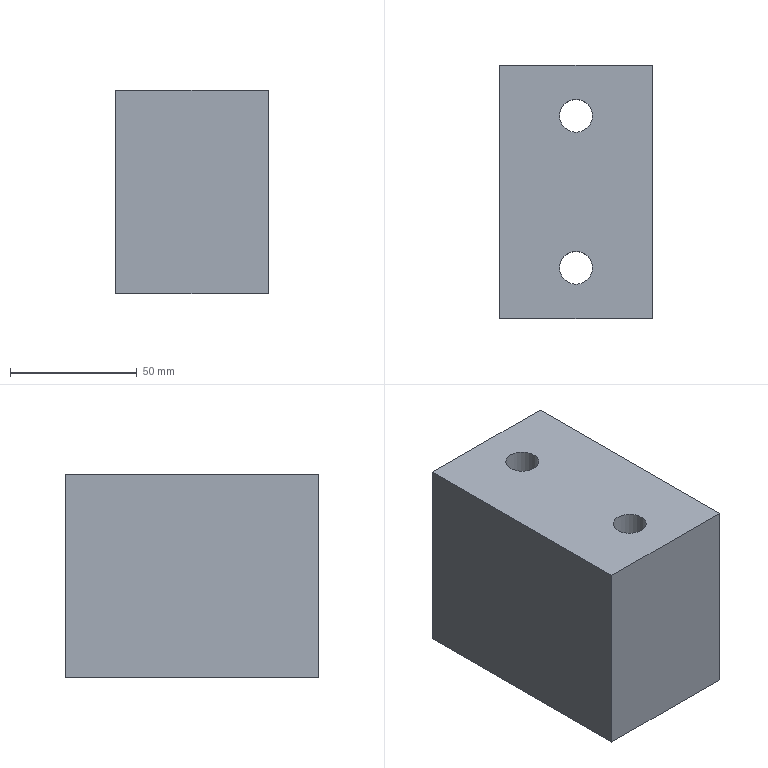Part | NX | features solid 2 | 1 solid | 12 faces | box 60 x 100 x 80.5 mm | volume 446935 mm3 | plane 8 | cylinder 4 | commonest cylinder face diameters 13 x2 20 x2
STEP:
#1=CARTESIAN_POINT('',(52.5,-343.5,48.));
#2=VERTEX_POINT('',#1);
#3=CARTESIAN_POINT('',(52.5,-350.,48.));
#4=DIRECTION('',(0.,0.,-1.));
#5=DIRECTION('',(0.,1.,0.));
#6=AXIS2_PLACEMENT_3D('',#3,#4,#5);
#7=CIRCLE('',#6,6.5);
#8=EDGE_CURVE('',#2,#2,#7,.T.);
#9=ORIENTED_EDGE('',*,*,#8,.F.);
#10=EDGE_LOOP('',(#9));
#11=FACE_BOUND('',#10,.T.);
#12=CARTESIAN_POINT('',(52.5,-340.,48.));
#13=VERTEX_POINT('',#12);
#14=CARTESIAN_POINT('',(52.5,-350.,48.));
#15=DIRECTION('',(0.,0.,-1.));
#16=DIRECTION('',(0.,1.,0.));
#17=AXIS2_PLACEMENT_3D('',#14,#15,#16);
#18=CIRCLE('',#17,10.);
#19=EDGE_CURVE('',#13,#13,#18,.T.);
#20=ORIENTED_EDGE('',*,*,#19,.T.);
#21=EDGE_LOOP('',(#20));
#22=FACE_BOUND('',#21,.T.);
#23=CARTESIAN_POINT('',(56.741,-346.137,48.));
#24=DIRECTION('',(0.,0.,1.));
#25=DIRECTION('',(0.,1.,0.));
#26=AXIS2_PLACEMENT_3D('',#23,#24,#25);
#27=PLANE('',#26);
#28=ADVANCED_FACE('',(#11,#22),#27,.F.);
#29=ORIENTED_EDGE('',*,*,#19,.F.);
#30=EDGE_LOOP('',(#29));
#31=FACE_BOUND('',#30,.T.);
#32=CARTESIAN_POINT('',(52.5,-340.,7.5));
#33=VERTEX_POINT('',#32);
#34=CARTESIAN_POINT('',(52.5,-350.,7.5));
#35=DIRECTION('',(0.,0.,-1.));
#36=DIRECTION('',(0.,1.,0.));
#37=AXIS2_PLACEMENT_3D('',#34,#35,#36);
#38=CIRCLE('',#37,10.);
#39=EDGE_CURVE('',#33,#33,#38,.F.);
#40=ORIENTED_EDGE('',*,*,#39,.F.);
#41=EDGE_LOOP('',(#40));
#42=FACE_BOUND('',#41,.T.);
#43=CARTESIAN_POINT('',(52.5,-350.,7.5));
#44=DIRECTION('',(0.,0.,1.));
#45=DIRECTION('',(0.,1.,0.));
#46=AXIS2_PLACEMENT_3D('',#43,#44,#45);
#47=CYLINDRICAL_SURFACE('',#46,10.);
#48=ADVANCED_FACE('',(#31,#42),#47,.F.);
#49=CARTESIAN_POINT('',(52.5,-343.5,88.));
#50=VERTEX_POINT('',#49);
#51=CARTESIAN_POINT('',(52.5,-350.,88.));
#52=DIRECTION('',(0.,0.,-1.));
#53=DIRECTION('',(0.,1.,0.));
#54=AXIS2_PLACEMENT_3D('',#51,#52,#53);
#55=CIRCLE('',#54,6.5);
#56=EDGE_CURVE('',#50,#50,#55,.T.);
#57=ORIENTED_EDGE('',*,*,#56,.F.);
#58=EDGE_LOOP('',(#57));
#59=FACE_BOUND('',#58,.T.);
#60=ORIENTED_EDGE('',*,*,#8,.T.);
#61=EDGE_LOOP('',(#60));
#62=FACE_BOUND('',#61,.T.);
#63=CARTESIAN_POINT('',(52.5,-350.,42.5));
#64=DIRECTION('',(0.,0.,1.));
#65=DIRECTION('',(0.,1.,0.));
#66=AXIS2_PLACEMENT_3D('',#63,#64,#65);
#67=CYLINDRICAL_SURFACE('',#66,6.5);
#68=ADVANCED_FACE('',(#59,#62),#67,.F.);
#69=CARTESIAN_POINT('',(52.5,-296.5,48.));
#70=VERTEX_POINT('',#69);
#71=CARTESIAN_POINT('',(52.5,-290.,48.));
#72=DIRECTION('',(0.,0.,1.));
#73=DIRECTION('',(0.,-1.,0.));
#74=AXIS2_PLACEMENT_3D('',#71,#72,#73);
#75=CIRCLE('',#74,6.5);
#76=EDGE_CURVE('',#70,#70,#75,.F.);
#77=ORIENTED_EDGE('',*,*,#76,.F.);
#78=EDGE_LOOP('',(#77));
#79=FACE_BOUND('',#78,.T.);
#80=CARTESIAN_POINT('',(52.5,-300.,48.));
#81=VERTEX_POINT('',#80);
#82=CARTESIAN_POINT('',(52.5,-290.,48.));
#83=DIRECTION('',(0.,0.,1.));
#84=DIRECTION('',(0.,-1.,0.));
#85=AXIS2_PLACEMENT_3D('',#82,#83,#84);
#86=CIRCLE('',#85,10.);
#87=EDGE_CURVE('',#81,#81,#86,.F.);
#88=ORIENTED_EDGE('',*,*,#87,.T.);
#89=EDGE_LOOP('',(#88));
#90=FACE_BOUND('',#89,.T.);
#91=CARTESIAN_POINT('',(56.741,-293.863,48.));
#92=DIRECTION('',(0.,0.,1.));
#93=DIRECTION('',(0.,-1.,0.));
#94=AXIS2_PLACEMENT_3D('',#91,#92,#93);
#95=PLANE('',#94);
#96=ADVANCED_FACE('',(#79,#90),#95,.F.);
#97=CARTESIAN_POINT('',(52.5,-296.5,88.));
#98=VERTEX_POINT('',#97);
#99=CARTESIAN_POINT('',(52.5,-290.,88.));
#100=DIRECTION('',(0.,0.,1.));
#101=DIRECTION('',(0.,-1.,0.));
#102=AXIS2_PLACEMENT_3D('',#99,#100,#101);
#103=CIRCLE('',#102,6.5);
#104=EDGE_CURVE('',#98,#98,#103,.F.);
#105=ORIENTED_EDGE('',*,*,#104,.F.);
#106=EDGE_LOOP('',(#105));
#107=FACE_BOUND('',#106,.T.);
#108=ORIENTED_EDGE('',*,*,#76,.T.);
#109=EDGE_LOOP('',(#108));
#110=FACE_BOUND('',#109,.T.);
#111=CARTESIAN_POINT('',(52.5,-290.,42.5));
#112=DIRECTION('',(0.,0.,1.));
#113=DIRECTION('',(0.,-1.,0.));
#114=AXIS2_PLACEMENT_3D('',#111,#112,#113);
#115=CYLINDRICAL_SURFACE('',#114,6.5);
#116=ADVANCED_FACE('',(#107,#110),#115,.F.);
#117=CARTESIAN_POINT('',(22.5,-370.,88.));
#118=VERTEX_POINT('',#117);
#119=CARTESIAN_POINT('',(22.5,-370.,7.5));
#120=VERTEX_POINT('',#119);
#121=CARTESIAN_POINT('',(22.5,-370.,88.));
#122=DIRECTION('',(0.,0.,-1.));
#123=VECTOR('',#122,1000.);
#124=LINE('',#121,#123);
#125=EDGE_CURVE('',#118,#120,#124,.T.);
#126=ORIENTED_EDGE('',*,*,#125,.T.);
#127=CARTESIAN_POINT('',(82.5,-370.,7.5));
#128=VERTEX_POINT('',#127);
#129=CARTESIAN_POINT('',(82.5,-370.,7.5));
#130=DIRECTION('',(1.,0.,0.));
#131=VECTOR('',#130,1000.);
#132=LINE('',#129,#131);
#133=EDGE_CURVE('',#120,#128,#132,.T.);
#134=ORIENTED_EDGE('',*,*,#133,.T.);
#135=CARTESIAN_POINT('',(82.5,-370.,88.));
#136=VERTEX_POINT('',#135);
#137=CARTESIAN_POINT('',(82.5,-370.,88.));
#138=DIRECTION('',(0.,0.,1.));
#139=VECTOR('',#138,1000.);
#140=LINE('',#137,#139);
#141=EDGE_CURVE('',#128,#136,#140,.T.);
#142=ORIENTED_EDGE('',*,*,#141,.T.);
#143=CARTESIAN_POINT('',(82.5,-370.,88.));
#144=DIRECTION('',(-1.,0.,0.));
#145=VECTOR('',#144,1000.);
#146=LINE('',#143,#145);
#147=EDGE_CURVE('',#136,#118,#146,.T.);
#148=ORIENTED_EDGE('',*,*,#147,.T.);
#149=EDGE_LOOP('',(#126,#134,#142,#148));
#150=FACE_BOUND('',#149,.T.);
#151=CARTESIAN_POINT('',(82.5,-370.,88.));
#152=DIRECTION('',(0.,-1.,0.));
#153=DIRECTION('',(0.,0.,-1.));
#154=AXIS2_PLACEMENT_3D('',#151,#152,#153);
#155=PLANE('',#154);
#156=ADVANCED_FACE('',(#150),#155,.T.);
#157=ORIENTED_EDGE('',*,*,#141,.F.);
#158=CARTESIAN_POINT('',(82.5,-270.,7.5));
#159=VERTEX_POINT('',#158);
#160=CARTESIAN_POINT('',(82.5,-300.,7.5));
#161=DIRECTION('',(0.,1.,0.));
#162=VECTOR('',#161,1000.);
#163=LINE('',#160,#162);
#164=EDGE_CURVE('',#128,#159,#163,.T.);
#165=ORIENTED_EDGE('',*,*,#164,.T.);
#166=CARTESIAN_POINT('',(82.5,-270.,88.));
#167=VERTEX_POINT('',#166);
#168=CARTESIAN_POINT('',(82.5,-270.,88.));
#169=DIRECTION('',(0.,0.,-1.));
#170=VECTOR('',#169,1000.);
#171=LINE('',#168,#170);
#172=EDGE_CURVE('',#167,#159,#171,.T.);
#173=ORIENTED_EDGE('',*,*,#172,.F.);
#174=CARTESIAN_POINT('',(82.5,-1209.121,88.));
#175=DIRECTION('',(0.,1.,0.));
#176=VECTOR('',#175,1000.);
#177=LINE('',#174,#176);
#178=EDGE_CURVE('',#136,#167,#177,.T.);
#179=ORIENTED_EDGE('',*,*,#178,.F.);
#180=EDGE_LOOP('',(#157,#165,#173,#179));
#181=FACE_BOUND('',#180,.T.);
#182=CARTESIAN_POINT('',(82.5,-300.,88.));
#183=DIRECTION('',(1.,0.,0.));
#184=DIRECTION('',(0.,0.,-1.));
#185=AXIS2_PLACEMENT_3D('',#182,#183,#184);
#186=PLANE('',#185);
#187=ADVANCED_FACE('',(#181),#186,.T.);
#188=ORIENTED_EDGE('',*,*,#172,.T.);
#189=CARTESIAN_POINT('',(22.5,-270.,7.5));
#190=VERTEX_POINT('',#189);
#191=CARTESIAN_POINT('',(82.5,-270.,7.5));
#192=DIRECTION('',(-1.,0.,0.));
#193=VECTOR('',#192,1000.);
#194=LINE('',#191,#193);
#195=EDGE_CURVE('',#159,#190,#194,.T.);
#196=ORIENTED_EDGE('',*,*,#195,.T.);
#197=CARTESIAN_POINT('',(22.5,-270.,88.));
#198=VERTEX_POINT('',#197);
#199=CARTESIAN_POINT('',(22.5,-270.,88.));
#200=DIRECTION('',(0.,0.,1.));
#201=VECTOR('',#200,1000.);
#202=LINE('',#199,#201);
#203=EDGE_CURVE('',#190,#198,#202,.T.);
#204=ORIENTED_EDGE('',*,*,#203,.T.);
#205=CARTESIAN_POINT('',(-302.5,-270.,88.));
#206=DIRECTION('',(-1.,0.,0.));
#207=VECTOR('',#206,1000.);
#208=LINE('',#205,#207);
#209=EDGE_CURVE('',#167,#198,#208,.T.);
#210=ORIENTED_EDGE('',*,*,#209,.F.);
#211=EDGE_LOOP('',(#188,#196,#204,#210));
#212=FACE_BOUND('',#211,.T.);
#213=CARTESIAN_POINT('',(82.5,-270.,88.));
#214=DIRECTION('',(0.,1.,0.));
#215=DIRECTION('',(0.,0.,1.));
#216=AXIS2_PLACEMENT_3D('',#213,#214,#215);
#217=PLANE('',#216);
#218=ADVANCED_FACE('',(#212),#217,.T.);
#219=ORIENTED_EDGE('',*,*,#203,.F.);
#220=CARTESIAN_POINT('',(22.5,-300.,7.5));
#221=DIRECTION('',(0.,-1.,0.));
#222=VECTOR('',#221,1000.);
#223=LINE('',#220,#222);
#224=EDGE_CURVE('',#190,#120,#223,.T.);
#225=ORIENTED_EDGE('',*,*,#224,.T.);
#226=ORIENTED_EDGE('',*,*,#125,.F.);
#227=CARTESIAN_POINT('',(22.5,-1209.121,88.));
#228=DIRECTION('',(0.,-1.,0.));
#229=VECTOR('',#228,1000.);
#230=LINE('',#227,#229);
#231=EDGE_CURVE('',#198,#118,#230,.T.);
#232=ORIENTED_EDGE('',*,*,#231,.F.);
#233=EDGE_LOOP('',(#219,#225,#226,#232));
#234=FACE_BOUND('',#233,.T.);
#235=CARTESIAN_POINT('',(22.5,-300.,88.));
#236=DIRECTION('',(-1.,0.,0.));
#237=DIRECTION('',(0.,0.,1.));
#238=AXIS2_PLACEMENT_3D('',#235,#236,#237);
#239=PLANE('',#238);
#240=ADVANCED_FACE('',(#234),#239,.T.);
#241=ORIENTED_EDGE('',*,*,#87,.F.);
#242=EDGE_LOOP('',(#241));
#243=FACE_BOUND('',#242,.T.);
#244=CARTESIAN_POINT('',(52.5,-300.,7.5));
#245=VERTEX_POINT('',#244);
#246=CARTESIAN_POINT('',(52.5,-290.,7.5));
#247=DIRECTION('',(0.,0.,1.));
#248=DIRECTION('',(0.,-1.,0.));
#249=AXIS2_PLACEMENT_3D('',#246,#247,#248);
#250=CIRCLE('',#249,10.);
#251=EDGE_CURVE('',#245,#245,#250,.T.);
#252=ORIENTED_EDGE('',*,*,#251,.F.);
#253=EDGE_LOOP('',(#252));
#254=FACE_BOUND('',#253,.T.);
#255=CARTESIAN_POINT('',(52.5,-290.,7.5));
#256=DIRECTION('',(0.,0.,1.));
#257=DIRECTION('',(0.,-1.,0.));
#258=AXIS2_PLACEMENT_3D('',#255,#256,#257);
#259=CYLINDRICAL_SURFACE('',#258,10.);
#260=ADVANCED_FACE('',(#243,#254),#259,.F.);
#261=ORIENTED_EDGE('',*,*,#39,.T.);
#262=EDGE_LOOP('',(#261));
#263=FACE_BOUND('',#262,.T.);
#264=ORIENTED_EDGE('',*,*,#251,.T.);
#265=EDGE_LOOP('',(#264));
#266=FACE_BOUND('',#265,.T.);
#267=ORIENTED_EDGE('',*,*,#224,.F.);
#268=ORIENTED_EDGE('',*,*,#195,.F.);
#269=ORIENTED_EDGE('',*,*,#164,.F.);
#270=ORIENTED_EDGE('',*,*,#133,.F.);
#271=EDGE_LOOP('',(#267,#268,#269,#270));
#272=FACE_BOUND('',#271,.T.);
#273=CARTESIAN_POINT('',(82.5,-370.,7.5));
#274=DIRECTION('',(0.,0.,-1.));
#275=DIRECTION('',(0.,1.,0.));
#276=AXIS2_PLACEMENT_3D('',#273,#274,#275);
#277=PLANE('',#276);
#278=ADVANCED_FACE('',(#263,#266,#272),#277,.T.);
#279=ORIENTED_EDGE('',*,*,#56,.T.);
#280=EDGE_LOOP('',(#279));
#281=FACE_BOUND('',#280,.T.);
#282=ORIENTED_EDGE('',*,*,#209,.T.);
#283=ORIENTED_EDGE('',*,*,#231,.T.);
#284=ORIENTED_EDGE('',*,*,#147,.F.);
#285=ORIENTED_EDGE('',*,*,#178,.T.);
#286=EDGE_LOOP('',(#282,#283,#284,#285));
#287=FACE_BOUND('',#286,.T.);
#288=ORIENTED_EDGE('',*,*,#104,.T.);
#289=EDGE_LOOP('',(#288));
#290=FACE_BOUND('',#289,.T.);
#291=CARTESIAN_POINT('',(-302.5,-1209.121,88.));
#292=DIRECTION('',(0.,0.,1.));
#293=DIRECTION('',(0.,-1.,0.));
#294=AXIS2_PLACEMENT_3D('',#291,#292,#293);
#295=PLANE('',#294);
#296=ADVANCED_FACE('',(#281,#287,#290),#295,.T.);
#297=CLOSED_SHELL('',(#28,#48,#68,#96,#116,#156,#187,#218,#240,#260,#278,#296));
#298=MANIFOLD_SOLID_BREP('',#297);
#299=(LENGTH_UNIT()NAMED_UNIT(*)SI_UNIT(.MILLI.,.METRE.));
#300=UNCERTAINTY_MEASURE_WITH_UNIT(LENGTH_MEASURE(0.00001),#299,'','');
#301=(NAMED_UNIT(*)PLANE_ANGLE_UNIT()SI_UNIT($,.RADIAN.));
#302=(NAMED_UNIT(*)SI_UNIT($,.STERADIAN.)SOLID_ANGLE_UNIT());
#303=(GEOMETRIC_REPRESENTATION_CONTEXT(3)GLOBAL_UNCERTAINTY_ASSIGNED_CONTEXT((#300))GLOBAL_UNIT_ASSIGNED_CONTEXT((#299,#301,#302))REPRESENTATION_CONTEXT('',''));
#304=ADVANCED_BREP_SHAPE_REPRESENTATION('',(#298),#303);